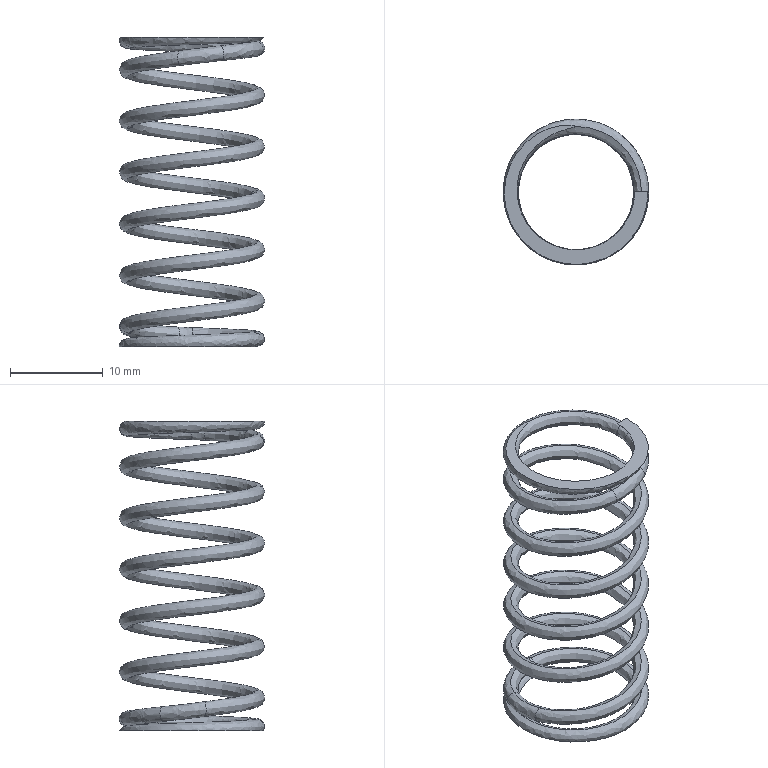Part | STEP file | 101000007889 | 1 solid | 22 faces | volume 638.551 mm3 | spline 18 | plane 4